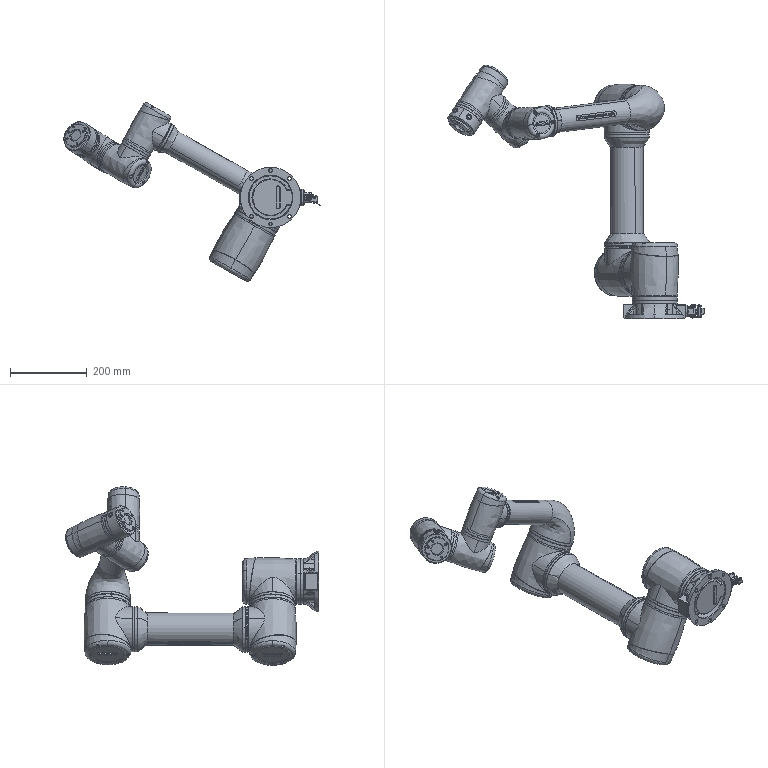Part | SolidWorks | features CoordSys 7, RefAxis 6, RefPoint 6, AEMSimFeature 1, Attribute 1 | 13 solids | 2035 faces | box 669.522 x 661.013 x 466.347 mm | volume 12326745 mm3 | plane 1082 | cylinder 457 | spline 354 | torus 80 | cone 59 | sphere 3 | commonest cylinder face diameters 118 x48 2 x43 1 x39 81 x38 0.4 x28 0.9 x24